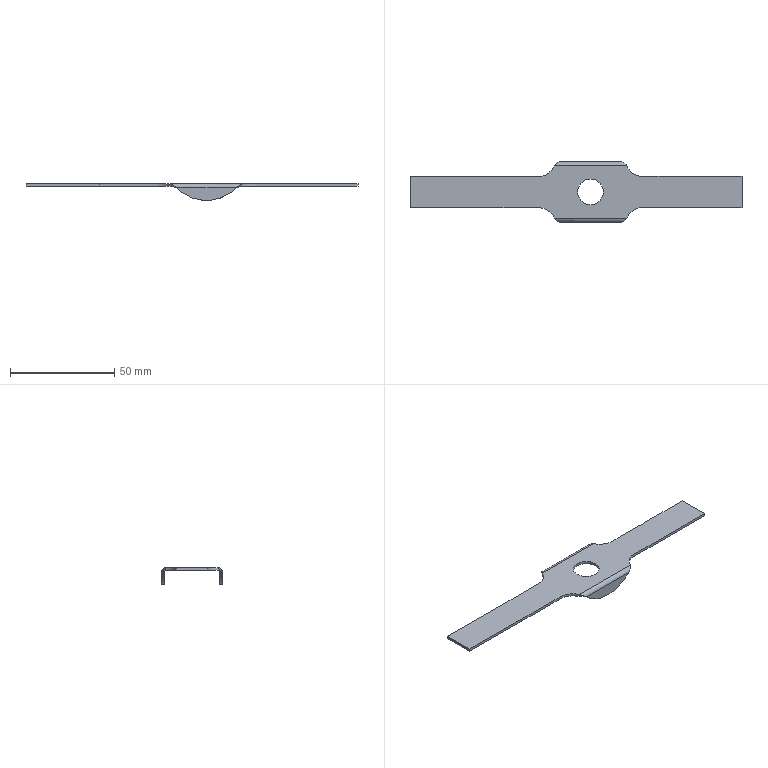Part | STEP file | gslz 2016.10.28-13_id1146_x_t | 1 solid | 26 faces | box 159.005 x 29 x 8 mm | volume 3787 mm3 | plane 10 | other 7 | cylinder 5 | spline 4 | commonest cylinder face diameters 1.5 x2 4 x2 12.3 x1